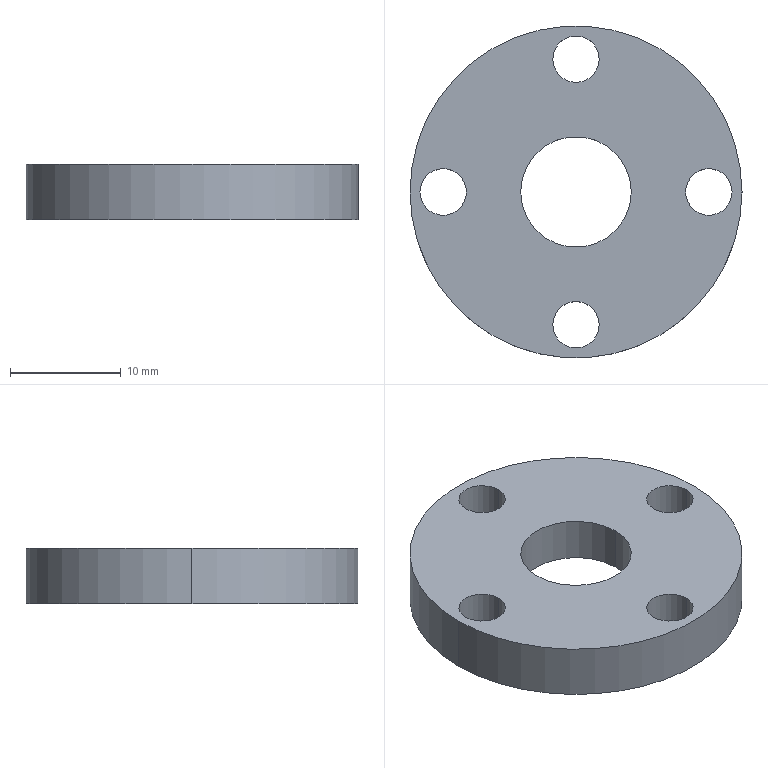Part | SolidWorks | features ICE 3, Chamfer 1, CirPattern 1, Extrusion 1 | 1 solid | 17 faces | box 30 x 30 x 5 mm | volume 2742 mm3 | cylinder 14 | plane 3 | commonest cylinder face diameters 4.2 x8 10 x2 16 x2 30 x2
STEP:
#1=CARTESIAN_POINT('',(5.,0.,1.));
#2=VERTEX_POINT('',#1);
#3=CARTESIAN_POINT('',(-5.,0.,1.));
#4=VERTEX_POINT('',#3);
#5=CARTESIAN_POINT('',(0.,0.,1.));
#6=DIRECTION('',(0.,0.,-1.));
#7=DIRECTION('',(-1.,0.,0.));
#8=AXIS2_PLACEMENT_3D('',#5,#6,#7);
#9=CIRCLE('',#8,5.);
#10=EDGE_CURVE('',#2,#4,#9,.T.);
#11=ORIENTED_EDGE('',*,*,#10,.T.);
#12=CARTESIAN_POINT('',(-5.,0.,5.));
#13=VERTEX_POINT('',#12);
#14=CARTESIAN_POINT('',(-5.,0.,0.));
#15=DIRECTION('',(0.,0.,1.));
#16=VECTOR('',#15,1000.);
#17=LINE('',#14,#16);
#18=EDGE_CURVE('',#4,#13,#17,.T.);
#19=ORIENTED_EDGE('',*,*,#18,.T.);
#20=CARTESIAN_POINT('',(5.,0.,5.));
#21=VERTEX_POINT('',#20);
#22=CARTESIAN_POINT('',(0.,0.,5.));
#23=DIRECTION('',(0.,0.,1.));
#24=DIRECTION('',(1.,0.,0.));
#25=AXIS2_PLACEMENT_3D('',#22,#23,#24);
#26=CIRCLE('',#25,5.);
#27=EDGE_CURVE('',#13,#21,#26,.T.);
#28=ORIENTED_EDGE('',*,*,#27,.T.);
#29=CARTESIAN_POINT('',(5.,0.,0.));
#30=DIRECTION('',(0.,0.,1.));
#31=VECTOR('',#30,1000.);
#32=LINE('',#29,#31);
#33=EDGE_CURVE('',#2,#21,#32,.T.);
#34=ORIENTED_EDGE('',*,*,#33,.F.);
#35=EDGE_LOOP('',(#11,#19,#28,#34));
#36=FACE_OUTER_BOUND('',#35,.T.);
#37=CARTESIAN_POINT('',(0.,0.,0.));
#38=DIRECTION('',(0.,0.,1.));
#39=DIRECTION('',(1.,0.,0.));
#40=AXIS2_PLACEMENT_3D('',#37,#38,#39);
#41=CYLINDRICAL_SURFACE('',#40,5.);
#42=ADVANCED_FACE('',(#36),#41,.F.);
#43=CARTESIAN_POINT('',(8.,0.,1.));
#44=VERTEX_POINT('',#43);
#45=CARTESIAN_POINT('',(-8.,0.,1.));
#46=VERTEX_POINT('',#45);
#47=CARTESIAN_POINT('',(0.,0.,1.));
#48=DIRECTION('',(0.,0.,-1.));
#49=DIRECTION('',(-1.,0.,0.));
#50=AXIS2_PLACEMENT_3D('',#47,#48,#49);
#51=CIRCLE('',#50,8.);
#52=EDGE_CURVE('',#44,#46,#51,.T.);
#53=ORIENTED_EDGE('',*,*,#52,.F.);
#54=CARTESIAN_POINT('',(8.,0.,0.));
#55=VERTEX_POINT('',#54);
#56=CARTESIAN_POINT('',(8.,0.,1.));
#57=DIRECTION('',(0.,0.,-1.));
#58=VECTOR('',#57,1000.);
#59=LINE('',#56,#58);
#60=EDGE_CURVE('',#44,#55,#59,.T.);
#61=ORIENTED_EDGE('',*,*,#60,.T.);
#62=CARTESIAN_POINT('',(-8.,0.,0.));
#63=VERTEX_POINT('',#62);
#64=CARTESIAN_POINT('',(0.,0.,0.));
#65=DIRECTION('',(0.,0.,-1.));
#66=DIRECTION('',(-1.,0.,0.));
#67=AXIS2_PLACEMENT_3D('',#64,#65,#66);
#68=CIRCLE('',#67,8.);
#69=EDGE_CURVE('',#55,#63,#68,.T.);
#70=ORIENTED_EDGE('',*,*,#69,.T.);
#71=CARTESIAN_POINT('',(-8.,0.,1.));
#72=DIRECTION('',(0.,0.,-1.));
#73=VECTOR('',#72,1000.);
#74=LINE('',#71,#73);
#75=EDGE_CURVE('',#46,#63,#74,.T.);
#76=ORIENTED_EDGE('',*,*,#75,.F.);
#77=EDGE_LOOP('',(#53,#61,#70,#76));
#78=FACE_OUTER_BOUND('',#77,.T.);
#79=CARTESIAN_POINT('',(0.,0.,1.));
#80=DIRECTION('',(0.,0.,-1.));
#81=DIRECTION('',(-1.,0.,0.));
#82=AXIS2_PLACEMENT_3D('',#79,#80,#81);
#83=CYLINDRICAL_SURFACE('',#82,8.);
#84=ADVANCED_FACE('',(#78),#83,.F.);
#85=CARTESIAN_POINT('',(9.9,0.,0.));
#86=VERTEX_POINT('',#85);
#87=CARTESIAN_POINT('',(14.1,0.,0.));
#88=VERTEX_POINT('',#87);
#89=CARTESIAN_POINT('',(12.,0.,0.));
#90=DIRECTION('',(0.,0.,1.));
#91=DIRECTION('',(0.,-1.,0.));
#92=AXIS2_PLACEMENT_3D('',#89,#90,#91);
#93=CIRCLE('',#92,2.1);
#94=EDGE_CURVE('',#86,#88,#93,.T.);
#95=ORIENTED_EDGE('',*,*,#94,.F.);
#96=CARTESIAN_POINT('',(9.9,0.,5.));
#97=VERTEX_POINT('',#96);
#98=CARTESIAN_POINT('',(9.9,0.,0.));
#99=DIRECTION('',(0.,0.,1.));
#100=VECTOR('',#99,1000.);
#101=LINE('',#98,#100);
#102=EDGE_CURVE('',#86,#97,#101,.T.);
#103=ORIENTED_EDGE('',*,*,#102,.T.);
#104=CARTESIAN_POINT('',(14.1,0.,5.));
#105=VERTEX_POINT('',#104);
#106=CARTESIAN_POINT('',(12.,0.,5.));
#107=DIRECTION('',(0.,0.,1.));
#108=DIRECTION('',(0.,-1.,0.));
#109=AXIS2_PLACEMENT_3D('',#106,#107,#108);
#110=CIRCLE('',#109,2.1);
#111=EDGE_CURVE('',#97,#105,#110,.T.);
#112=ORIENTED_EDGE('',*,*,#111,.T.);
#113=CARTESIAN_POINT('',(14.1,0.,0.));
#114=DIRECTION('',(0.,0.,1.));
#115=VECTOR('',#114,1000.);
#116=LINE('',#113,#115);
#117=EDGE_CURVE('',#88,#105,#116,.T.);
#118=ORIENTED_EDGE('',*,*,#117,.F.);
#119=EDGE_LOOP('',(#95,#103,#112,#118));
#120=FACE_OUTER_BOUND('',#119,.T.);
#121=CARTESIAN_POINT('',(12.,0.,0.));
#122=DIRECTION('',(0.,0.,1.));
#123=DIRECTION('',(1.,0.,0.));
#124=AXIS2_PLACEMENT_3D('',#121,#122,#123);
#125=CYLINDRICAL_SURFACE('',#124,2.1);
#126=ADVANCED_FACE('',(#120),#125,.F.);
#127=CARTESIAN_POINT('',(-2.1,-12.,0.));
#128=VERTEX_POINT('',#127);
#129=CARTESIAN_POINT('',(2.1,-12.,0.));
#130=VERTEX_POINT('',#129);
#131=CARTESIAN_POINT('',(0.,-12.,0.));
#132=DIRECTION('',(0.,0.,1.));
#133=DIRECTION('',(-1.,0.,0.));
#134=AXIS2_PLACEMENT_3D('',#131,#132,#133);
#135=CIRCLE('',#134,2.1);
#136=EDGE_CURVE('',#128,#130,#135,.T.);
#137=ORIENTED_EDGE('',*,*,#136,.F.);
#138=CARTESIAN_POINT('',(-2.1,-12.,5.));
#139=VERTEX_POINT('',#138);
#140=CARTESIAN_POINT('',(-2.1,-12.,0.));
#141=DIRECTION('',(0.,0.,1.));
#142=VECTOR('',#141,1000.);
#143=LINE('',#140,#142);
#144=EDGE_CURVE('',#128,#139,#143,.T.);
#145=ORIENTED_EDGE('',*,*,#144,.T.);
#146=CARTESIAN_POINT('',(2.1,-12.,5.));
#147=VERTEX_POINT('',#146);
#148=CARTESIAN_POINT('',(0.,-12.,5.));
#149=DIRECTION('',(0.,0.,1.));
#150=DIRECTION('',(-1.,0.,0.));
#151=AXIS2_PLACEMENT_3D('',#148,#149,#150);
#152=CIRCLE('',#151,2.1);
#153=EDGE_CURVE('',#139,#147,#152,.T.);
#154=ORIENTED_EDGE('',*,*,#153,.T.);
#155=CARTESIAN_POINT('',(2.1,-12.,0.));
#156=DIRECTION('',(0.,0.,1.));
#157=VECTOR('',#156,1000.);
#158=LINE('',#155,#157);
#159=EDGE_CURVE('',#130,#147,#158,.T.);
#160=ORIENTED_EDGE('',*,*,#159,.F.);
#161=EDGE_LOOP('',(#137,#145,#154,#160));
#162=FACE_OUTER_BOUND('',#161,.T.);
#163=CARTESIAN_POINT('',(0.,-12.,0.));
#164=DIRECTION('',(0.,0.,1.));
#165=DIRECTION('',(1.,0.,0.));
#166=AXIS2_PLACEMENT_3D('',#163,#164,#165);
#167=CYLINDRICAL_SURFACE('',#166,2.1);
#168=ADVANCED_FACE('',(#162),#167,.F.);
#169=CARTESIAN_POINT('',(-14.1,0.,0.));
#170=VERTEX_POINT('',#169);
#171=CARTESIAN_POINT('',(-9.9,0.,0.));
#172=VERTEX_POINT('',#171);
#173=CARTESIAN_POINT('',(-12.,0.,0.));
#174=DIRECTION('',(0.,0.,1.));
#175=DIRECTION('',(0.,1.,0.));
#176=AXIS2_PLACEMENT_3D('',#173,#174,#175);
#177=CIRCLE('',#176,2.1);
#178=EDGE_CURVE('',#170,#172,#177,.T.);
#179=ORIENTED_EDGE('',*,*,#178,.F.);
#180=CARTESIAN_POINT('',(-14.1,0.,5.));
#181=VERTEX_POINT('',#180);
#182=CARTESIAN_POINT('',(-14.1,0.,0.));
#183=DIRECTION('',(0.,0.,1.));
#184=VECTOR('',#183,1000.);
#185=LINE('',#182,#184);
#186=EDGE_CURVE('',#170,#181,#185,.T.);
#187=ORIENTED_EDGE('',*,*,#186,.T.);
#188=CARTESIAN_POINT('',(-9.9,0.,5.));
#189=VERTEX_POINT('',#188);
#190=CARTESIAN_POINT('',(-12.,0.,5.));
#191=DIRECTION('',(0.,0.,1.));
#192=DIRECTION('',(0.,1.,0.));
#193=AXIS2_PLACEMENT_3D('',#190,#191,#192);
#194=CIRCLE('',#193,2.1);
#195=EDGE_CURVE('',#181,#189,#194,.T.);
#196=ORIENTED_EDGE('',*,*,#195,.T.);
#197=CARTESIAN_POINT('',(-9.9,0.,0.));
#198=DIRECTION('',(0.,0.,1.));
#199=VECTOR('',#198,1000.);
#200=LINE('',#197,#199);
#201=EDGE_CURVE('',#172,#189,#200,.T.);
#202=ORIENTED_EDGE('',*,*,#201,.F.);
#203=EDGE_LOOP('',(#179,#187,#196,#202));
#204=FACE_OUTER_BOUND('',#203,.T.);
#205=CARTESIAN_POINT('',(-12.,0.,0.));
#206=DIRECTION('',(0.,0.,1.));
#207=DIRECTION('',(1.,0.,0.));
#208=AXIS2_PLACEMENT_3D('',#205,#206,#207);
#209=CYLINDRICAL_SURFACE('',#208,2.1);
#210=ADVANCED_FACE('',(#204),#209,.F.);
#211=CARTESIAN_POINT('',(-2.1,12.,0.));
#212=VERTEX_POINT('',#211);
#213=CARTESIAN_POINT('',(2.1,12.,0.));
#214=VERTEX_POINT('',#213);
#215=CARTESIAN_POINT('',(0.,12.,0.));
#216=DIRECTION('',(0.,0.,1.));
#217=DIRECTION('',(1.,0.,0.));
#218=AXIS2_PLACEMENT_3D('',#215,#216,#217);
#219=CIRCLE('',#218,2.1);
#220=EDGE_CURVE('',#212,#214,#219,.T.);
#221=ORIENTED_EDGE('',*,*,#220,.F.);
#222=CARTESIAN_POINT('',(-2.1,12.,5.));
#223=VERTEX_POINT('',#222);
#224=CARTESIAN_POINT('',(-2.1,12.,0.));
#225=DIRECTION('',(0.,0.,1.));
#226=VECTOR('',#225,1000.);
#227=LINE('',#224,#226);
#228=EDGE_CURVE('',#212,#223,#227,.T.);
#229=ORIENTED_EDGE('',*,*,#228,.T.);
#230=CARTESIAN_POINT('',(2.1,12.,5.));
#231=VERTEX_POINT('',#230);
#232=CARTESIAN_POINT('',(0.,12.,5.));
#233=DIRECTION('',(0.,0.,1.));
#234=DIRECTION('',(1.,0.,0.));
#235=AXIS2_PLACEMENT_3D('',#232,#233,#234);
#236=CIRCLE('',#235,2.1);
#237=EDGE_CURVE('',#223,#231,#236,.T.);
#238=ORIENTED_EDGE('',*,*,#237,.T.);
#239=CARTESIAN_POINT('',(2.1,12.,0.));
#240=DIRECTION('',(0.,0.,1.));
#241=VECTOR('',#240,1000.);
#242=LINE('',#239,#241);
#243=EDGE_CURVE('',#214,#231,#242,.T.);
#244=ORIENTED_EDGE('',*,*,#243,.F.);
#245=EDGE_LOOP('',(#221,#229,#238,#244));
#246=FACE_OUTER_BOUND('',#245,.T.);
#247=CARTESIAN_POINT('',(0.,12.,0.));
#248=DIRECTION('',(0.,0.,1.));
#249=DIRECTION('',(1.,0.,0.));
#250=AXIS2_PLACEMENT_3D('',#247,#248,#249);
#251=CYLINDRICAL_SURFACE('',#250,2.1);
#252=ADVANCED_FACE('',(#246),#251,.F.);
#253=CARTESIAN_POINT('',(15.,0.,5.));
#254=VERTEX_POINT('',#253);
#255=CARTESIAN_POINT('',(-15.,0.,5.));
#256=VERTEX_POINT('',#255);
#257=CARTESIAN_POINT('',(0.,0.,5.));
#258=DIRECTION('',(0.,0.,1.));
#259=DIRECTION('',(1.,0.,0.));
#260=AXIS2_PLACEMENT_3D('',#257,#258,#259);
#261=CIRCLE('',#260,15.);
#262=EDGE_CURVE('',#254,#256,#261,.T.);
#263=ORIENTED_EDGE('',*,*,#262,.F.);
#264=CARTESIAN_POINT('',(15.,0.,0.));
#265=VERTEX_POINT('',#264);
#266=CARTESIAN_POINT('',(15.,0.,5.));
#267=DIRECTION('',(0.,0.,-1.));
#268=VECTOR('',#267,1000.);
#269=LINE('',#266,#268);
#270=EDGE_CURVE('',#254,#265,#269,.T.);
#271=ORIENTED_EDGE('',*,*,#270,.T.);
#272=CARTESIAN_POINT('',(-15.,0.,0.));
#273=VERTEX_POINT('',#272);
#274=CARTESIAN_POINT('',(0.,0.,0.));
#275=DIRECTION('',(0.,0.,1.));
#276=DIRECTION('',(1.,0.,0.));
#277=AXIS2_PLACEMENT_3D('',#274,#275,#276);
#278=CIRCLE('',#277,15.);
#279=EDGE_CURVE('',#265,#273,#278,.T.);
#280=ORIENTED_EDGE('',*,*,#279,.T.);
#281=CARTESIAN_POINT('',(-15.,0.,5.));
#282=DIRECTION('',(0.,0.,-1.));
#283=VECTOR('',#282,1000.);
#284=LINE('',#281,#283);
#285=EDGE_CURVE('',#256,#273,#284,.T.);
#286=ORIENTED_EDGE('',*,*,#285,.F.);
#287=EDGE_LOOP('',(#263,#271,#280,#286));
#288=FACE_OUTER_BOUND('',#287,.T.);
#289=CARTESIAN_POINT('',(0.,0.,5.));
#290=DIRECTION('',(0.,0.,-1.));
#291=DIRECTION('',(-1.,0.,0.));
#292=AXIS2_PLACEMENT_3D('',#289,#290,#291);
#293=CYLINDRICAL_SURFACE('',#292,15.);
#294=ADVANCED_FACE('',(#288),#293,.T.);
#295=ORIENTED_EDGE('',*,*,#270,.F.);
#296=CARTESIAN_POINT('',(0.,0.,5.));
#297=DIRECTION('',(0.,0.,1.));
#298=DIRECTION('',(1.,0.,0.));
#299=AXIS2_PLACEMENT_3D('',#296,#297,#298);
#300=CIRCLE('',#299,15.);
#301=EDGE_CURVE('',#256,#254,#300,.T.);
#302=ORIENTED_EDGE('',*,*,#301,.F.);
#303=ORIENTED_EDGE('',*,*,#285,.T.);
#304=CARTESIAN_POINT('',(0.,0.,0.));
#305=DIRECTION('',(0.,0.,1.));
#306=DIRECTION('',(1.,0.,0.));
#307=AXIS2_PLACEMENT_3D('',#304,#305,#306);
#308=CIRCLE('',#307,15.);
#309=EDGE_CURVE('',#273,#265,#308,.T.);
#310=ORIENTED_EDGE('',*,*,#309,.T.);
#311=EDGE_LOOP('',(#295,#302,#303,#310));
#312=FACE_OUTER_BOUND('',#311,.T.);
#313=CARTESIAN_POINT('',(0.,0.,5.));
#314=DIRECTION('',(0.,0.,-1.));
#315=DIRECTION('',(-1.,0.,0.));
#316=AXIS2_PLACEMENT_3D('',#313,#314,#315);
#317=CYLINDRICAL_SURFACE('',#316,15.);
#318=ADVANCED_FACE('',(#312),#317,.T.);
#319=CARTESIAN_POINT('',(0.,0.,5.));
#320=DIRECTION('',(0.,0.,1.));
#321=DIRECTION('',(1.,0.,0.));
#322=AXIS2_PLACEMENT_3D('',#319,#320,#321);
#323=CIRCLE('',#322,5.);
#324=EDGE_CURVE('',#21,#13,#323,.T.);
#325=ORIENTED_EDGE('',*,*,#324,.F.);
#326=ORIENTED_EDGE('',*,*,#27,.F.);
#327=EDGE_LOOP('',(#325,#326));
#328=FACE_BOUND('',#327,.T.);
#329=CARTESIAN_POINT('',(12.,0.,5.));
#330=DIRECTION('',(0.,0.,1.));
#331=DIRECTION('',(0.,-1.,0.));
#332=AXIS2_PLACEMENT_3D('',#329,#330,#331);
#333=CIRCLE('',#332,2.1);
#334=EDGE_CURVE('',#105,#97,#333,.T.);
#335=ORIENTED_EDGE('',*,*,#334,.F.);
#336=ORIENTED_EDGE('',*,*,#111,.F.);
#337=EDGE_LOOP('',(#335,#336));
#338=FACE_BOUND('',#337,.T.);
#339=CARTESIAN_POINT('',(0.,-12.,5.));
#340=DIRECTION('',(0.,0.,1.));
#341=DIRECTION('',(-1.,0.,0.));
#342=AXIS2_PLACEMENT_3D('',#339,#340,#341);
#343=CIRCLE('',#342,2.1);
#344=EDGE_CURVE('',#147,#139,#343,.T.);
#345=ORIENTED_EDGE('',*,*,#344,.F.);
#346=ORIENTED_EDGE('',*,*,#153,.F.);
#347=EDGE_LOOP('',(#345,#346));
#348=FACE_BOUND('',#347,.T.);
#349=CARTESIAN_POINT('',(-12.,0.,5.));
#350=DIRECTION('',(0.,0.,1.));
#351=DIRECTION('',(0.,1.,0.));
#352=AXIS2_PLACEMENT_3D('',#349,#350,#351);
#353=CIRCLE('',#352,2.1);
#354=EDGE_CURVE('',#189,#181,#353,.T.);
#355=ORIENTED_EDGE('',*,*,#354,.F.);
#356=ORIENTED_EDGE('',*,*,#195,.F.);
#357=EDGE_LOOP('',(#355,#356));
#358=FACE_BOUND('',#357,.T.);
#359=CARTESIAN_POINT('',(0.,12.,5.));
#360=DIRECTION('',(0.,0.,1.));
#361=DIRECTION('',(1.,0.,0.));
#362=AXIS2_PLACEMENT_3D('',#359,#360,#361);
#363=CIRCLE('',#362,2.1);
#364=EDGE_CURVE('',#231,#223,#363,.T.);
#365=ORIENTED_EDGE('',*,*,#364,.F.);
#366=ORIENTED_EDGE('',*,*,#237,.F.);
#367=EDGE_LOOP('',(#365,#366));
#368=FACE_BOUND('',#367,.T.);
#369=ORIENTED_EDGE('',*,*,#301,.T.);
#370=ORIENTED_EDGE('',*,*,#262,.T.);
#371=EDGE_LOOP('',(#369,#370));
#372=FACE_OUTER_BOUND('',#371,.T.);
#373=CARTESIAN_POINT('',(0.,0.,5.));
#374=DIRECTION('',(0.,0.,1.));
#375=DIRECTION('',(1.,0.,0.));
#376=AXIS2_PLACEMENT_3D('',#373,#374,#375);
#377=PLANE('',#376);
#378=ADVANCED_FACE('',(#328,#338,#348,#358,#368,#372),#377,.T.);
#379=CARTESIAN_POINT('',(0.,0.,0.));
#380=DIRECTION('',(0.,0.,-1.));
#381=DIRECTION('',(-1.,0.,0.));
#382=AXIS2_PLACEMENT_3D('',#379,#380,#381);
#383=CIRCLE('',#382,8.);
#384=EDGE_CURVE('',#63,#55,#383,.T.);
#385=ORIENTED_EDGE('',*,*,#384,.F.);
#386=ORIENTED_EDGE('',*,*,#69,.F.);
#387=EDGE_LOOP('',(#385,#386));
#388=FACE_BOUND('',#387,.T.);
#389=CARTESIAN_POINT('',(12.,0.,0.));
#390=DIRECTION('',(0.,0.,1.));
#391=DIRECTION('',(0.,-1.,0.));
#392=AXIS2_PLACEMENT_3D('',#389,#390,#391);
#393=CIRCLE('',#392,2.1);
#394=EDGE_CURVE('',#88,#86,#393,.T.);
#395=ORIENTED_EDGE('',*,*,#394,.T.);
#396=ORIENTED_EDGE('',*,*,#94,.T.);
#397=EDGE_LOOP('',(#395,#396));
#398=FACE_BOUND('',#397,.T.);
#399=CARTESIAN_POINT('',(0.,-12.,0.));
#400=DIRECTION('',(0.,0.,1.));
#401=DIRECTION('',(-1.,0.,0.));
#402=AXIS2_PLACEMENT_3D('',#399,#400,#401);
#403=CIRCLE('',#402,2.1);
#404=EDGE_CURVE('',#130,#128,#403,.T.);
#405=ORIENTED_EDGE('',*,*,#404,.T.);
#406=ORIENTED_EDGE('',*,*,#136,.T.);
#407=EDGE_LOOP('',(#405,#406));
#408=FACE_BOUND('',#407,.T.);
#409=CARTESIAN_POINT('',(-12.,0.,0.));
#410=DIRECTION('',(0.,0.,1.));
#411=DIRECTION('',(0.,1.,0.));
#412=AXIS2_PLACEMENT_3D('',#409,#410,#411);
#413=CIRCLE('',#412,2.1);
#414=EDGE_CURVE('',#172,#170,#413,.T.);
#415=ORIENTED_EDGE('',*,*,#414,.T.);
#416=ORIENTED_EDGE('',*,*,#178,.T.);
#417=EDGE_LOOP('',(#415,#416));
#418=FACE_BOUND('',#417,.T.);
#419=CARTESIAN_POINT('',(0.,12.,0.));
#420=DIRECTION('',(0.,0.,1.));
#421=DIRECTION('',(1.,0.,0.));
#422=AXIS2_PLACEMENT_3D('',#419,#420,#421);
#423=CIRCLE('',#422,2.1);
#424=EDGE_CURVE('',#214,#212,#423,.T.);
#425=ORIENTED_EDGE('',*,*,#424,.T.);
#426=ORIENTED_EDGE('',*,*,#220,.T.);
#427=EDGE_LOOP('',(#425,#426));
#428=FACE_BOUND('',#427,.T.);
#429=ORIENTED_EDGE('',*,*,#309,.F.);
#430=ORIENTED_EDGE('',*,*,#279,.F.);
#431=EDGE_LOOP('',(#429,#430));
#432=FACE_OUTER_BOUND('',#431,.T.);
#433=CARTESIAN_POINT('',(0.,0.,0.));
#434=DIRECTION('',(0.,0.,1.));
#435=DIRECTION('',(1.,0.,0.));
#436=AXIS2_PLACEMENT_3D('',#433,#434,#435);
#437=PLANE('',#436);
#438=ADVANCED_FACE('',(#388,#398,#408,#418,#428,#432),#437,.F.);
#439=ORIENTED_EDGE('',*,*,#228,.F.);
#440=ORIENTED_EDGE('',*,*,#424,.F.);
#441=ORIENTED_EDGE('',*,*,#243,.T.);
#442=ORIENTED_EDGE('',*,*,#364,.T.);
#443=EDGE_LOOP('',(#439,#440,#441,#442));
#444=FACE_OUTER_BOUND('',#443,.T.);
#445=CARTESIAN_POINT('',(0.,12.,0.));
#446=DIRECTION('',(0.,0.,1.));
#447=DIRECTION('',(1.,0.,0.));
#448=AXIS2_PLACEMENT_3D('',#445,#446,#447);
#449=CYLINDRICAL_SURFACE('',#448,2.1);
#450=ADVANCED_FACE('',(#444),#449,.F.);
#451=ORIENTED_EDGE('',*,*,#186,.F.);
#452=ORIENTED_EDGE('',*,*,#414,.F.);
#453=ORIENTED_EDGE('',*,*,#201,.T.);
#454=ORIENTED_EDGE('',*,*,#354,.T.);
#455=EDGE_LOOP('',(#451,#452,#453,#454));
#456=FACE_OUTER_BOUND('',#455,.T.);
#457=CARTESIAN_POINT('',(-12.,0.,0.));
#458=DIRECTION('',(0.,0.,1.));
#459=DIRECTION('',(1.,0.,0.));
#460=AXIS2_PLACEMENT_3D('',#457,#458,#459);
#461=CYLINDRICAL_SURFACE('',#460,2.1);
#462=ADVANCED_FACE('',(#456),#461,.F.);
#463=ORIENTED_EDGE('',*,*,#144,.F.);
#464=ORIENTED_EDGE('',*,*,#404,.F.);
#465=ORIENTED_EDGE('',*,*,#159,.T.);
#466=ORIENTED_EDGE('',*,*,#344,.T.);
#467=EDGE_LOOP('',(#463,#464,#465,#466));
#468=FACE_OUTER_BOUND('',#467,.T.);
#469=CARTESIAN_POINT('',(0.,-12.,0.));
#470=DIRECTION('',(0.,0.,1.));
#471=DIRECTION('',(1.,0.,0.));
#472=AXIS2_PLACEMENT_3D('',#469,#470,#471);
#473=CYLINDRICAL_SURFACE('',#472,2.1);
#474=ADVANCED_FACE('',(#468),#473,.F.);
#475=ORIENTED_EDGE('',*,*,#102,.F.);
#476=ORIENTED_EDGE('',*,*,#394,.F.);
#477=ORIENTED_EDGE('',*,*,#117,.T.);
#478=ORIENTED_EDGE('',*,*,#334,.T.);
#479=EDGE_LOOP('',(#475,#476,#477,#478));
#480=FACE_OUTER_BOUND('',#479,.T.);
#481=CARTESIAN_POINT('',(12.,0.,0.));
#482=DIRECTION('',(0.,0.,1.));
#483=DIRECTION('',(1.,0.,0.));
#484=AXIS2_PLACEMENT_3D('',#481,#482,#483);
#485=CYLINDRICAL_SURFACE('',#484,2.1);
#486=ADVANCED_FACE('',(#480),#485,.F.);
#487=ORIENTED_EDGE('',*,*,#60,.F.);
#488=CARTESIAN_POINT('',(0.,0.,1.));
#489=DIRECTION('',(0.,0.,-1.));
#490=DIRECTION('',(-1.,0.,0.));
#491=AXIS2_PLACEMENT_3D('',#488,#489,#490);
#492=CIRCLE('',#491,8.);
#493=EDGE_CURVE('',#46,#44,#492,.T.);
#494=ORIENTED_EDGE('',*,*,#493,.F.);
#495=ORIENTED_EDGE('',*,*,#75,.T.);
#496=ORIENTED_EDGE('',*,*,#384,.T.);
#497=EDGE_LOOP('',(#487,#494,#495,#496));
#498=FACE_OUTER_BOUND('',#497,.T.);
#499=CARTESIAN_POINT('',(0.,0.,1.));
#500=DIRECTION('',(0.,0.,-1.));
#501=DIRECTION('',(-1.,0.,0.));
#502=AXIS2_PLACEMENT_3D('',#499,#500,#501);
#503=CYLINDRICAL_SURFACE('',#502,8.);
#504=ADVANCED_FACE('',(#498),#503,.F.);
#505=ORIENTED_EDGE('',*,*,#10,.F.);
#506=CARTESIAN_POINT('',(0.,0.,1.));
#507=DIRECTION('',(0.,0.,-1.));
#508=DIRECTION('',(-1.,0.,0.));
#509=AXIS2_PLACEMENT_3D('',#506,#507,#508);
#510=CIRCLE('',#509,5.);
#511=EDGE_CURVE('',#4,#2,#510,.T.);
#512=ORIENTED_EDGE('',*,*,#511,.F.);
#513=EDGE_LOOP('',(#505,#512));
#514=FACE_BOUND('',#513,.T.);
#515=ORIENTED_EDGE('',*,*,#493,.T.);
#516=ORIENTED_EDGE('',*,*,#52,.T.);
#517=EDGE_LOOP('',(#515,#516));
#518=FACE_OUTER_BOUND('',#517,.T.);
#519=CARTESIAN_POINT('',(0.,0.,1.));
#520=DIRECTION('',(0.,0.,-1.));
#521=DIRECTION('',(-1.,0.,0.));
#522=AXIS2_PLACEMENT_3D('',#519,#520,#521);
#523=PLANE('',#522);
#524=ADVANCED_FACE('',(#514,#518),#523,.T.);
#525=ORIENTED_EDGE('',*,*,#18,.F.);
#526=ORIENTED_EDGE('',*,*,#511,.T.);
#527=ORIENTED_EDGE('',*,*,#33,.T.);
#528=ORIENTED_EDGE('',*,*,#324,.T.);
#529=EDGE_LOOP('',(#525,#526,#527,#528));
#530=FACE_OUTER_BOUND('',#529,.T.);
#531=CARTESIAN_POINT('',(0.,0.,0.));
#532=DIRECTION('',(0.,0.,1.));
#533=DIRECTION('',(1.,0.,0.));
#534=AXIS2_PLACEMENT_3D('',#531,#532,#533);
#535=CYLINDRICAL_SURFACE('',#534,5.);
#536=ADVANCED_FACE('',(#530),#535,.F.);
#537=CLOSED_SHELL('',(#42,#84,#126,#168,#210,#252,#294,#318,#378,#438,#450,#462,#474,#486,#504,#524,#536));
#538=MANIFOLD_SOLID_BREP('',#537);
#539=CARTESIAN_POINT('',(0.,0.,0.));
#540=DIRECTION('',(0.,0.,1.));
#541=DIRECTION('',(1.,0.,0.));
#542=AXIS2_PLACEMENT_3D('',#539,#540,#541);
#543=(LENGTH_UNIT()NAMED_UNIT(*)SI_UNIT(.MILLI.,.METRE.));
#544=UNCERTAINTY_MEASURE_WITH_UNIT(LENGTH_MEASURE(0.00001),#543,'','');
#545=(NAMED_UNIT(*)PLANE_ANGLE_UNIT()SI_UNIT($,.RADIAN.));
#546=(NAMED_UNIT(*)SI_UNIT($,.STERADIAN.)SOLID_ANGLE_UNIT());
#547=(GEOMETRIC_REPRESENTATION_CONTEXT(3)GLOBAL_UNCERTAINTY_ASSIGNED_CONTEXT((#544))GLOBAL_UNIT_ASSIGNED_CONTEXT((#543,#545,#546))REPRESENTATION_CONTEXT('',''));
#548=ADVANCED_BREP_SHAPE_REPRESENTATION('',(#538,#542),#547);